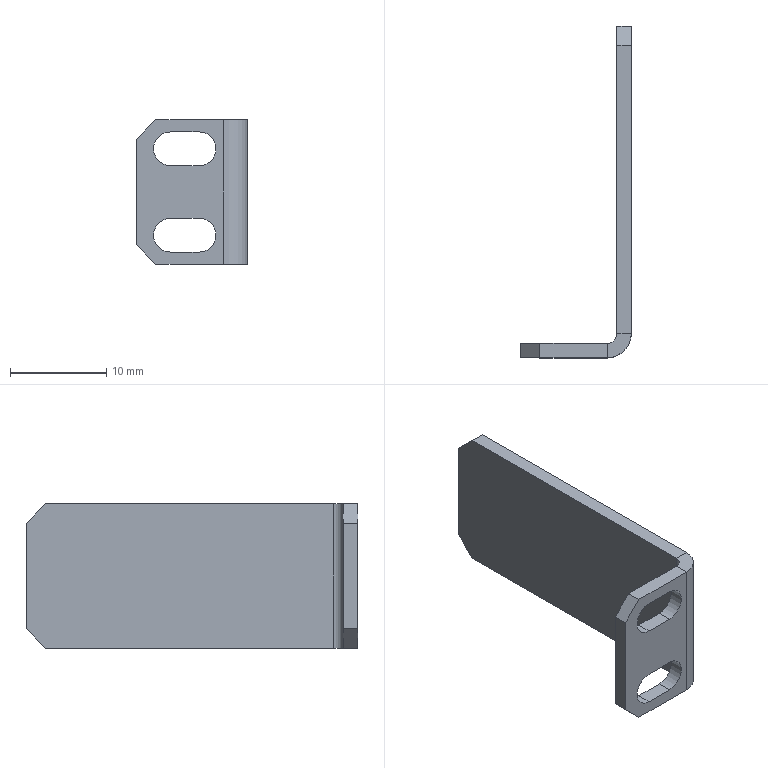Part | NX | 1 solid | 26 faces | box 11.5 x 34.5 x 15 mm | volume 911.987 mm3 | plane 20 | cylinder 6 | commonest cylinder face diameters 3.5 x4 2 x1 5 x1
STEP:
#1=CARTESIAN_POINT('',(4.,-1.5,-7.5));
#2=VERTEX_POINT('',#1);
#3=CARTESIAN_POINT('',(-3.,-1.5,-7.5));
#4=VERTEX_POINT('',#3);
#5=CARTESIAN_POINT('',(-5.,-1.5,-7.5));
#6=DIRECTION('',(-1.,0.,0.));
#7=VECTOR('',#6,1000.);
#8=LINE('',#5,#7);
#9=EDGE_CURVE('',#2,#4,#8,.T.);
#10=ORIENTED_EDGE('',*,*,#9,.T.);
#11=CARTESIAN_POINT('',(-3.,0.,-7.5));
#12=VERTEX_POINT('',#11);
#13=CARTESIAN_POINT('',(-3.,-1.5,-7.5));
#14=DIRECTION('',(0.,1.,0.));
#15=VECTOR('',#14,1000.);
#16=LINE('',#13,#15);
#17=EDGE_CURVE('',#4,#12,#16,.T.);
#18=ORIENTED_EDGE('',*,*,#17,.T.);
#19=CARTESIAN_POINT('',(4.,0.,-7.5));
#20=VERTEX_POINT('',#19);
#21=CARTESIAN_POINT('',(-5.,0.,-7.5));
#22=DIRECTION('',(-1.,0.,0.));
#23=VECTOR('',#22,1000.);
#24=LINE('',#21,#23);
#25=EDGE_CURVE('',#20,#12,#24,.T.);
#26=ORIENTED_EDGE('',*,*,#25,.F.);
#27=CARTESIAN_POINT('',(4.,0.,-7.5));
#28=DIRECTION('',(0.,-1.,0.));
#29=VECTOR('',#28,1000.);
#30=LINE('',#27,#29);
#31=EDGE_CURVE('',#20,#2,#30,.T.);
#32=ORIENTED_EDGE('',*,*,#31,.T.);
#33=EDGE_LOOP('',(#10,#18,#26,#32));
#34=FACE_BOUND('',#33,.T.);
#35=CARTESIAN_POINT('',(-5.,-1.5,-7.5));
#36=DIRECTION('',(0.,0.,-1.));
#37=DIRECTION('',(-1.,0.,0.));
#38=AXIS2_PLACEMENT_3D('',#35,#36,#37);
#39=PLANE('',#38);
#40=ADVANCED_FACE('',(#34),#39,.T.);
#41=CARTESIAN_POINT('',(-1.5,-1.5,6.25));
#42=VERTEX_POINT('',#41);
#43=CARTESIAN_POINT('',(-1.5,-1.5,2.75));
#44=VERTEX_POINT('',#43);
#45=CARTESIAN_POINT('',(-1.5,-1.5,4.5));
#46=DIRECTION('',(0.,-1.,0.));
#47=DIRECTION('',(0.,0.,-1.));
#48=AXIS2_PLACEMENT_3D('',#45,#46,#47);
#49=CIRCLE('',#48,1.75);
#50=EDGE_CURVE('',#42,#44,#49,.T.);
#51=ORIENTED_EDGE('',*,*,#50,.F.);
#52=CARTESIAN_POINT('',(1.5,-1.5,6.25));
#53=VERTEX_POINT('',#52);
#54=CARTESIAN_POINT('',(-1.5,-1.5,6.25));
#55=DIRECTION('',(-1.,0.,0.));
#56=VECTOR('',#55,1000.);
#57=LINE('',#54,#56);
#58=EDGE_CURVE('',#53,#42,#57,.T.);
#59=ORIENTED_EDGE('',*,*,#58,.F.);
#60=CARTESIAN_POINT('',(1.5,-1.5,2.75));
#61=VERTEX_POINT('',#60);
#62=CARTESIAN_POINT('',(1.5,-1.5,4.5));
#63=DIRECTION('',(0.,-1.,0.));
#64=DIRECTION('',(0.,0.,-1.));
#65=AXIS2_PLACEMENT_3D('',#62,#63,#64);
#66=CIRCLE('',#65,1.75);
#67=EDGE_CURVE('',#61,#53,#66,.T.);
#68=ORIENTED_EDGE('',*,*,#67,.F.);
#69=CARTESIAN_POINT('',(-1.5,-1.5,2.75));
#70=DIRECTION('',(1.,0.,0.));
#71=VECTOR('',#70,1000.);
#72=LINE('',#69,#71);
#73=EDGE_CURVE('',#44,#61,#72,.T.);
#74=ORIENTED_EDGE('',*,*,#73,.F.);
#75=EDGE_LOOP('',(#51,#59,#68,#74));
#76=FACE_BOUND('',#75,.T.);
#77=CARTESIAN_POINT('',(-1.5,-1.5,-2.75));
#78=VERTEX_POINT('',#77);
#79=CARTESIAN_POINT('',(-1.5,-1.5,-6.25));
#80=VERTEX_POINT('',#79);
#81=CARTESIAN_POINT('',(-1.5,-1.5,-4.5));
#82=DIRECTION('',(0.,-1.,0.));
#83=DIRECTION('',(0.,0.,-1.));
#84=AXIS2_PLACEMENT_3D('',#81,#82,#83);
#85=CIRCLE('',#84,1.75);
#86=EDGE_CURVE('',#78,#80,#85,.T.);
#87=ORIENTED_EDGE('',*,*,#86,.F.);
#88=CARTESIAN_POINT('',(1.5,-1.5,-2.75));
#89=VERTEX_POINT('',#88);
#90=CARTESIAN_POINT('',(-1.5,-1.5,-2.75));
#91=DIRECTION('',(-1.,0.,0.));
#92=VECTOR('',#91,1000.);
#93=LINE('',#90,#92);
#94=EDGE_CURVE('',#89,#78,#93,.T.);
#95=ORIENTED_EDGE('',*,*,#94,.F.);
#96=CARTESIAN_POINT('',(1.5,-1.5,-6.25));
#97=VERTEX_POINT('',#96);
#98=CARTESIAN_POINT('',(1.5,-1.5,-4.5));
#99=DIRECTION('',(0.,-1.,0.));
#100=DIRECTION('',(0.,0.,-1.));
#101=AXIS2_PLACEMENT_3D('',#98,#99,#100);
#102=CIRCLE('',#101,1.75);
#103=EDGE_CURVE('',#97,#89,#102,.T.);
#104=ORIENTED_EDGE('',*,*,#103,.F.);
#105=CARTESIAN_POINT('',(-1.5,-1.5,-6.25));
#106=DIRECTION('',(1.,0.,0.));
#107=VECTOR('',#106,1000.);
#108=LINE('',#105,#107);
#109=EDGE_CURVE('',#80,#97,#108,.T.);
#110=ORIENTED_EDGE('',*,*,#109,.F.);
#111=EDGE_LOOP('',(#87,#95,#104,#110));
#112=FACE_BOUND('',#111,.T.);
#113=CARTESIAN_POINT('',(-3.,-1.5,7.5));
#114=VERTEX_POINT('',#113);
#115=CARTESIAN_POINT('',(4.,-1.5,7.5));
#116=VERTEX_POINT('',#115);
#117=CARTESIAN_POINT('',(-5.,-1.5,7.5));
#118=DIRECTION('',(1.,0.,0.));
#119=VECTOR('',#118,1000.);
#120=LINE('',#117,#119);
#121=EDGE_CURVE('',#114,#116,#120,.T.);
#122=ORIENTED_EDGE('',*,*,#121,.F.);
#123=CARTESIAN_POINT('',(-5.,-1.5,5.5));
#124=VERTEX_POINT('',#123);
#125=CARTESIAN_POINT('',(-5.25,-1.5,5.25));
#126=DIRECTION('',(0.7071,0.,0.7071));
#127=VECTOR('',#126,1000.);
#128=LINE('',#125,#127);
#129=EDGE_CURVE('',#114,#124,#128,.F.);
#130=ORIENTED_EDGE('',*,*,#129,.T.);
#131=CARTESIAN_POINT('',(-5.,-1.5,-5.5));
#132=VERTEX_POINT('',#131);
#133=CARTESIAN_POINT('',(-5.,-1.5,7.5));
#134=DIRECTION('',(0.,0.,1.));
#135=VECTOR('',#134,1000.);
#136=LINE('',#133,#135);
#137=EDGE_CURVE('',#132,#124,#136,.T.);
#138=ORIENTED_EDGE('',*,*,#137,.F.);
#139=CARTESIAN_POINT('',(-5.25,-1.5,-5.25));
#140=DIRECTION('',(-0.7071,0.,0.7071));
#141=VECTOR('',#140,1000.);
#142=LINE('',#139,#141);
#143=EDGE_CURVE('',#132,#4,#142,.F.);
#144=ORIENTED_EDGE('',*,*,#143,.T.);
#145=ORIENTED_EDGE('',*,*,#9,.F.);
#146=CARTESIAN_POINT('',(4.,-1.5,-7.5));
#147=DIRECTION('',(0.,0.,-1.));
#148=VECTOR('',#147,1000.);
#149=LINE('',#146,#148);
#150=EDGE_CURVE('',#2,#116,#149,.F.);
#151=ORIENTED_EDGE('',*,*,#150,.T.);
#152=EDGE_LOOP('',(#122,#130,#138,#144,#145,#151));
#153=FACE_BOUND('',#152,.T.);
#154=CARTESIAN_POINT('',(0.,-1.5,0.));
#155=DIRECTION('',(0.,-1.,0.));
#156=DIRECTION('',(0.,0.,-1.));
#157=AXIS2_PLACEMENT_3D('',#154,#155,#156);
#158=PLANE('',#157);
#159=ADVANCED_FACE('',(#76,#112,#153),#158,.T.);
#160=CARTESIAN_POINT('',(1.5,0.,6.25));
#161=VERTEX_POINT('',#160);
#162=CARTESIAN_POINT('',(-1.5,0.,6.25));
#163=VERTEX_POINT('',#162);
#164=CARTESIAN_POINT('',(0.,0.,6.25));
#165=DIRECTION('',(-1.,0.,0.));
#166=VECTOR('',#165,1000.);
#167=LINE('',#164,#166);
#168=EDGE_CURVE('',#161,#163,#167,.T.);
#169=ORIENTED_EDGE('',*,*,#168,.T.);
#170=CARTESIAN_POINT('',(-1.5,0.,2.75));
#171=VERTEX_POINT('',#170);
#172=CARTESIAN_POINT('',(-1.5,0.,4.5));
#173=DIRECTION('',(0.,-1.,0.));
#174=DIRECTION('',(0.,0.,-1.));
#175=AXIS2_PLACEMENT_3D('',#172,#173,#174);
#176=CIRCLE('',#175,1.75);
#177=EDGE_CURVE('',#163,#171,#176,.T.);
#178=ORIENTED_EDGE('',*,*,#177,.T.);
#179=CARTESIAN_POINT('',(1.5,0.,2.75));
#180=VERTEX_POINT('',#179);
#181=CARTESIAN_POINT('',(0.,0.,2.75));
#182=DIRECTION('',(1.,0.,0.));
#183=VECTOR('',#182,1000.);
#184=LINE('',#181,#183);
#185=EDGE_CURVE('',#171,#180,#184,.T.);
#186=ORIENTED_EDGE('',*,*,#185,.T.);
#187=CARTESIAN_POINT('',(1.5,0.,4.5));
#188=DIRECTION('',(0.,-1.,0.));
#189=DIRECTION('',(0.,0.,-1.));
#190=AXIS2_PLACEMENT_3D('',#187,#188,#189);
#191=CIRCLE('',#190,1.75);
#192=EDGE_CURVE('',#180,#161,#191,.T.);
#193=ORIENTED_EDGE('',*,*,#192,.T.);
#194=EDGE_LOOP('',(#169,#178,#186,#193));
#195=FACE_BOUND('',#194,.T.);
#196=CARTESIAN_POINT('',(1.5,0.,-2.75));
#197=VERTEX_POINT('',#196);
#198=CARTESIAN_POINT('',(-1.5,0.,-2.75));
#199=VERTEX_POINT('',#198);
#200=CARTESIAN_POINT('',(0.,0.,-2.75));
#201=DIRECTION('',(-1.,0.,0.));
#202=VECTOR('',#201,1000.);
#203=LINE('',#200,#202);
#204=EDGE_CURVE('',#197,#199,#203,.T.);
#205=ORIENTED_EDGE('',*,*,#204,.T.);
#206=CARTESIAN_POINT('',(-1.5,0.,-6.25));
#207=VERTEX_POINT('',#206);
#208=CARTESIAN_POINT('',(-1.5,0.,-4.5));
#209=DIRECTION('',(0.,-1.,0.));
#210=DIRECTION('',(0.,0.,-1.));
#211=AXIS2_PLACEMENT_3D('',#208,#209,#210);
#212=CIRCLE('',#211,1.75);
#213=EDGE_CURVE('',#199,#207,#212,.T.);
#214=ORIENTED_EDGE('',*,*,#213,.T.);
#215=CARTESIAN_POINT('',(1.5,0.,-6.25));
#216=VERTEX_POINT('',#215);
#217=CARTESIAN_POINT('',(0.,0.,-6.25));
#218=DIRECTION('',(1.,0.,0.));
#219=VECTOR('',#218,1000.);
#220=LINE('',#217,#219);
#221=EDGE_CURVE('',#207,#216,#220,.T.);
#222=ORIENTED_EDGE('',*,*,#221,.T.);
#223=CARTESIAN_POINT('',(1.5,0.,-4.5));
#224=DIRECTION('',(0.,-1.,0.));
#225=DIRECTION('',(0.,0.,-1.));
#226=AXIS2_PLACEMENT_3D('',#223,#224,#225);
#227=CIRCLE('',#226,1.75);
#228=EDGE_CURVE('',#216,#197,#227,.T.);
#229=ORIENTED_EDGE('',*,*,#228,.T.);
#230=EDGE_LOOP('',(#205,#214,#222,#229));
#231=FACE_BOUND('',#230,.T.);
#232=CARTESIAN_POINT('',(-5.,0.,-5.5));
#233=VERTEX_POINT('',#232);
#234=CARTESIAN_POINT('',(-5.,0.,5.5));
#235=VERTEX_POINT('',#234);
#236=CARTESIAN_POINT('',(-5.,0.,7.5));
#237=DIRECTION('',(0.,0.,1.));
#238=VECTOR('',#237,1000.);
#239=LINE('',#236,#238);
#240=EDGE_CURVE('',#233,#235,#239,.T.);
#241=ORIENTED_EDGE('',*,*,#240,.T.);
#242=CARTESIAN_POINT('',(-3.,0.,7.5));
#243=VERTEX_POINT('',#242);
#244=CARTESIAN_POINT('',(-5.,0.,5.5));
#245=DIRECTION('',(-0.7071,0.,-0.7071));
#246=VECTOR('',#245,1000.);
#247=LINE('',#244,#246);
#248=EDGE_CURVE('',#235,#243,#247,.F.);
#249=ORIENTED_EDGE('',*,*,#248,.T.);
#250=CARTESIAN_POINT('',(4.,0.,7.5));
#251=VERTEX_POINT('',#250);
#252=CARTESIAN_POINT('',(-5.,0.,7.5));
#253=DIRECTION('',(1.,0.,0.));
#254=VECTOR('',#253,1000.);
#255=LINE('',#252,#254);
#256=EDGE_CURVE('',#243,#251,#255,.T.);
#257=ORIENTED_EDGE('',*,*,#256,.T.);
#258=CARTESIAN_POINT('',(4.,0.,-7.5));
#259=DIRECTION('',(0.,0.,-1.));
#260=VECTOR('',#259,1000.);
#261=LINE('',#258,#260);
#262=EDGE_CURVE('',#20,#251,#261,.F.);
#263=ORIENTED_EDGE('',*,*,#262,.F.);
#264=ORIENTED_EDGE('',*,*,#25,.T.);
#265=CARTESIAN_POINT('',(-3.,0.,-7.5));
#266=DIRECTION('',(0.7071,0.,-0.7071));
#267=VECTOR('',#266,1000.);
#268=LINE('',#265,#267);
#269=EDGE_CURVE('',#12,#233,#268,.F.);
#270=ORIENTED_EDGE('',*,*,#269,.T.);
#271=EDGE_LOOP('',(#241,#249,#257,#263,#264,#270));
#272=FACE_BOUND('',#271,.T.);
#273=CARTESIAN_POINT('',(0.,0.,0.));
#274=DIRECTION('',(0.,-1.,0.));
#275=DIRECTION('',(0.,0.,-1.));
#276=AXIS2_PLACEMENT_3D('',#273,#274,#275);
#277=PLANE('',#276);
#278=ADVANCED_FACE('',(#195,#231,#272),#277,.F.);
#279=ORIENTED_EDGE('',*,*,#256,.F.);
#280=CARTESIAN_POINT('',(-3.,-1.5,7.5));
#281=DIRECTION('',(0.,-1.,0.));
#282=VECTOR('',#281,1000.);
#283=LINE('',#280,#282);
#284=EDGE_CURVE('',#243,#114,#283,.T.);
#285=ORIENTED_EDGE('',*,*,#284,.T.);
#286=ORIENTED_EDGE('',*,*,#121,.T.);
#287=CARTESIAN_POINT('',(4.,0.,7.5));
#288=DIRECTION('',(0.,-1.,0.));
#289=VECTOR('',#288,1000.);
#290=LINE('',#287,#289);
#291=EDGE_CURVE('',#251,#116,#290,.T.);
#292=ORIENTED_EDGE('',*,*,#291,.F.);
#293=EDGE_LOOP('',(#279,#285,#286,#292));
#294=FACE_BOUND('',#293,.T.);
#295=CARTESIAN_POINT('',(-5.,-1.5,7.5));
#296=DIRECTION('',(0.,0.,1.));
#297=DIRECTION('',(1.,0.,0.));
#298=AXIS2_PLACEMENT_3D('',#295,#296,#297);
#299=PLANE('',#298);
#300=ADVANCED_FACE('',(#294),#299,.T.);
#301=ORIENTED_EDGE('',*,*,#137,.T.);
#302=CARTESIAN_POINT('',(-5.,-1.5,5.5));
#303=DIRECTION('',(0.,1.,0.));
#304=VECTOR('',#303,1000.);
#305=LINE('',#302,#304);
#306=EDGE_CURVE('',#124,#235,#305,.T.);
#307=ORIENTED_EDGE('',*,*,#306,.T.);
#308=ORIENTED_EDGE('',*,*,#240,.F.);
#309=CARTESIAN_POINT('',(-5.,-1.5,-5.5));
#310=DIRECTION('',(0.,-1.,0.));
#311=VECTOR('',#310,1000.);
#312=LINE('',#309,#311);
#313=EDGE_CURVE('',#233,#132,#312,.T.);
#314=ORIENTED_EDGE('',*,*,#313,.T.);
#315=EDGE_LOOP('',(#301,#307,#308,#314));
#316=FACE_BOUND('',#315,.T.);
#317=CARTESIAN_POINT('',(-5.,-1.5,7.5));
#318=DIRECTION('',(-1.,0.,0.));
#319=DIRECTION('',(0.,0.,1.));
#320=AXIS2_PLACEMENT_3D('',#317,#318,#319);
#321=PLANE('',#320);
#322=ADVANCED_FACE('',(#316),#321,.T.);
#323=CARTESIAN_POINT('',(5.,1.,7.5));
#324=VERTEX_POINT('',#323);
#325=CARTESIAN_POINT('',(6.5,1.,7.5));
#326=VERTEX_POINT('',#325);
#327=CARTESIAN_POINT('',(5.,1.,7.5));
#328=DIRECTION('',(1.,0.,0.));
#329=VECTOR('',#328,1000.);
#330=LINE('',#327,#329);
#331=EDGE_CURVE('',#324,#326,#330,.T.);
#332=ORIENTED_EDGE('',*,*,#331,.F.);
#333=CARTESIAN_POINT('',(4.,1.,7.5));
#334=DIRECTION('',(0.,0.,-1.));
#335=DIRECTION('',(-1.,0.,0.));
#336=AXIS2_PLACEMENT_3D('',#333,#334,#335);
#337=CIRCLE('',#336,1.);
#338=EDGE_CURVE('',#251,#324,#337,.F.);
#339=ORIENTED_EDGE('',*,*,#338,.F.);
#340=ORIENTED_EDGE('',*,*,#291,.T.);
#341=CARTESIAN_POINT('',(4.,1.,7.5));
#342=DIRECTION('',(0.,0.,-1.));
#343=DIRECTION('',(-1.,0.,0.));
#344=AXIS2_PLACEMENT_3D('',#341,#342,#343);
#345=CIRCLE('',#344,2.5);
#346=EDGE_CURVE('',#116,#326,#345,.F.);
#347=ORIENTED_EDGE('',*,*,#346,.T.);
#348=EDGE_LOOP('',(#332,#339,#340,#347));
#349=FACE_BOUND('',#348,.T.);
#350=CARTESIAN_POINT('',(4.,1.,7.5));
#351=DIRECTION('',(0.,0.,1.));
#352=DIRECTION('',(1.,0.,0.));
#353=AXIS2_PLACEMENT_3D('',#350,#351,#352);
#354=PLANE('',#353);
#355=ADVANCED_FACE('',(#349),#354,.T.);
#356=CARTESIAN_POINT('',(5.,1.,-7.5));
#357=VERTEX_POINT('',#356);
#358=CARTESIAN_POINT('',(4.,1.,-7.5));
#359=DIRECTION('',(0.,0.,-1.));
#360=DIRECTION('',(-1.,0.,0.));
#361=AXIS2_PLACEMENT_3D('',#358,#359,#360);
#362=CIRCLE('',#361,1.);
#363=EDGE_CURVE('',#357,#20,#362,.T.);
#364=ORIENTED_EDGE('',*,*,#363,.F.);
#365=CARTESIAN_POINT('',(6.5,1.,-7.5));
#366=VERTEX_POINT('',#365);
#367=CARTESIAN_POINT('',(5.,1.,-7.5));
#368=DIRECTION('',(1.,0.,0.));
#369=VECTOR('',#368,1000.);
#370=LINE('',#367,#369);
#371=EDGE_CURVE('',#357,#366,#370,.T.);
#372=ORIENTED_EDGE('',*,*,#371,.T.);
#373=CARTESIAN_POINT('',(4.,1.,-7.5));
#374=DIRECTION('',(0.,0.,-1.));
#375=DIRECTION('',(-1.,0.,0.));
#376=AXIS2_PLACEMENT_3D('',#373,#374,#375);
#377=CIRCLE('',#376,2.5);
#378=EDGE_CURVE('',#366,#2,#377,.T.);
#379=ORIENTED_EDGE('',*,*,#378,.T.);
#380=ORIENTED_EDGE('',*,*,#31,.F.);
#381=EDGE_LOOP('',(#364,#372,#379,#380));
#382=FACE_BOUND('',#381,.T.);
#383=CARTESIAN_POINT('',(4.,1.,-7.5));
#384=DIRECTION('',(0.,0.,1.));
#385=DIRECTION('',(1.,0.,0.));
#386=AXIS2_PLACEMENT_3D('',#383,#384,#385);
#387=PLANE('',#386);
#388=ADVANCED_FACE('',(#382),#387,.F.);
#389=ORIENTED_EDGE('',*,*,#150,.F.);
#390=ORIENTED_EDGE('',*,*,#378,.F.);
#391=CARTESIAN_POINT('',(6.5,1.,0.));
#392=DIRECTION('',(0.,0.,1.));
#393=VECTOR('',#392,1000.);
#394=LINE('',#391,#393);
#395=EDGE_CURVE('',#366,#326,#394,.T.);
#396=ORIENTED_EDGE('',*,*,#395,.T.);
#397=ORIENTED_EDGE('',*,*,#346,.F.);
#398=EDGE_LOOP('',(#389,#390,#396,#397));
#399=FACE_BOUND('',#398,.T.);
#400=CARTESIAN_POINT('',(4.,1.,-7.5));
#401=DIRECTION('',(0.,0.,-1.));
#402=DIRECTION('',(1.,0.,0.));
#403=AXIS2_PLACEMENT_3D('',#400,#401,#402);
#404=CYLINDRICAL_SURFACE('',#403,2.5);
#405=ADVANCED_FACE('',(#399),#404,.T.);
#406=ORIENTED_EDGE('',*,*,#262,.T.);
#407=ORIENTED_EDGE('',*,*,#338,.T.);
#408=CARTESIAN_POINT('',(5.,1.,7.5));
#409=DIRECTION('',(0.,0.,-1.));
#410=VECTOR('',#409,1000.);
#411=LINE('',#408,#410);
#412=EDGE_CURVE('',#324,#357,#411,.T.);
#413=ORIENTED_EDGE('',*,*,#412,.T.);
#414=ORIENTED_EDGE('',*,*,#363,.T.);
#415=EDGE_LOOP('',(#406,#407,#413,#414));
#416=FACE_BOUND('',#415,.T.);
#417=CARTESIAN_POINT('',(4.,1.,-7.5));
#418=DIRECTION('',(0.,0.,-1.));
#419=DIRECTION('',(1.,0.,0.));
#420=AXIS2_PLACEMENT_3D('',#417,#418,#419);
#421=CYLINDRICAL_SURFACE('',#420,1.);
#422=ADVANCED_FACE('',(#416),#421,.F.);
#423=CARTESIAN_POINT('',(6.5,31.,7.5));
#424=VERTEX_POINT('',#423);
#425=CARTESIAN_POINT('',(6.5,0.,7.5));
#426=DIRECTION('',(0.,-1.,0.));
#427=VECTOR('',#426,1000.);
#428=LINE('',#425,#427);
#429=EDGE_CURVE('',#424,#326,#428,.T.);
#430=ORIENTED_EDGE('',*,*,#429,.F.);
#431=CARTESIAN_POINT('',(5.,31.,7.5));
#432=VERTEX_POINT('',#431);
#433=CARTESIAN_POINT('',(6.5,31.,7.5));
#434=DIRECTION('',(-1.,0.,0.));
#435=VECTOR('',#434,1000.);
#436=LINE('',#433,#435);
#437=EDGE_CURVE('',#424,#432,#436,.T.);
#438=ORIENTED_EDGE('',*,*,#437,.T.);
#439=CARTESIAN_POINT('',(5.,0.,7.5));
#440=DIRECTION('',(0.,-1.,0.));
#441=VECTOR('',#440,1000.);
#442=LINE('',#439,#441);
#443=EDGE_CURVE('',#432,#324,#442,.T.);
#444=ORIENTED_EDGE('',*,*,#443,.T.);
#445=ORIENTED_EDGE('',*,*,#331,.T.);
#446=EDGE_LOOP('',(#430,#438,#444,#445));
#447=FACE_BOUND('',#446,.T.);
#448=CARTESIAN_POINT('',(6.5,0.,7.5));
#449=DIRECTION('',(0.,0.,-1.));
#450=DIRECTION('',(0.,1.,0.));
#451=AXIS2_PLACEMENT_3D('',#448,#449,#450);
#452=PLANE('',#451);
#453=ADVANCED_FACE('',(#447),#452,.F.);
#454=CARTESIAN_POINT('',(5.,31.,-7.5));
#455=VERTEX_POINT('',#454);
#456=CARTESIAN_POINT('',(5.,33.,-7.5));
#457=DIRECTION('',(0.,1.,0.));
#458=VECTOR('',#457,1000.);
#459=LINE('',#456,#458);
#460=EDGE_CURVE('',#357,#455,#459,.T.);
#461=ORIENTED_EDGE('',*,*,#460,.T.);
#462=CARTESIAN_POINT('',(6.5,31.,-7.5));
#463=VERTEX_POINT('',#462);
#464=CARTESIAN_POINT('',(6.5,31.,-7.5));
#465=DIRECTION('',(1.,0.,0.));
#466=VECTOR('',#465,1000.);
#467=LINE('',#464,#466);
#468=EDGE_CURVE('',#455,#463,#467,.T.);
#469=ORIENTED_EDGE('',*,*,#468,.T.);
#470=CARTESIAN_POINT('',(6.5,33.,-7.5));
#471=DIRECTION('',(0.,1.,0.));
#472=VECTOR('',#471,1000.);
#473=LINE('',#470,#472);
#474=EDGE_CURVE('',#366,#463,#473,.T.);
#475=ORIENTED_EDGE('',*,*,#474,.F.);
#476=ORIENTED_EDGE('',*,*,#371,.F.);
#477=EDGE_LOOP('',(#461,#469,#475,#476));
#478=FACE_BOUND('',#477,.T.);
#479=CARTESIAN_POINT('',(6.5,33.,-7.5));
#480=DIRECTION('',(0.,0.,1.));
#481=DIRECTION('',(0.,-1.,0.));
#482=AXIS2_PLACEMENT_3D('',#479,#480,#481);
#483=PLANE('',#482);
#484=ADVANCED_FACE('',(#478),#483,.F.);
#485=CARTESIAN_POINT('',(6.5,33.,-5.5));
#486=VERTEX_POINT('',#485);
#487=CARTESIAN_POINT('',(6.5,33.,5.5));
#488=VERTEX_POINT('',#487);
#489=CARTESIAN_POINT('',(6.5,33.,7.5));
#490=DIRECTION('',(0.,0.,1.));
#491=VECTOR('',#490,1000.);
#492=LINE('',#489,#491);
#493=EDGE_CURVE('',#486,#488,#492,.T.);
#494=ORIENTED_EDGE('',*,*,#493,.T.);
#495=CARTESIAN_POINT('',(6.5,31.,7.5));
#496=DIRECTION('',(0.,0.7071,-0.7071));
#497=VECTOR('',#496,1000.);
#498=LINE('',#495,#497);
#499=EDGE_CURVE('',#488,#424,#498,.F.);
#500=ORIENTED_EDGE('',*,*,#499,.T.);
#501=ORIENTED_EDGE('',*,*,#429,.T.);
#502=ORIENTED_EDGE('',*,*,#395,.F.);
#503=ORIENTED_EDGE('',*,*,#474,.T.);
#504=CARTESIAN_POINT('',(6.5,33.,-5.5));
#505=DIRECTION('',(0.,-0.7071,-0.7071));
#506=VECTOR('',#505,1000.);
#507=LINE('',#504,#506);
#508=EDGE_CURVE('',#463,#486,#507,.F.);
#509=ORIENTED_EDGE('',*,*,#508,.T.);
#510=EDGE_LOOP('',(#494,#500,#501,#502,#503,#509));
#511=FACE_BOUND('',#510,.T.);
#512=CARTESIAN_POINT('',(6.5,0.,0.));
#513=DIRECTION('',(-1.,0.,0.));
#514=DIRECTION('',(0.,-1.,0.));
#515=AXIS2_PLACEMENT_3D('',#512,#513,#514);
#516=PLANE('',#515);
#517=ADVANCED_FACE('',(#511),#516,.F.);
#518=ORIENTED_EDGE('',*,*,#443,.F.);
#519=CARTESIAN_POINT('',(5.,33.,5.5));
#520=VERTEX_POINT('',#519);
#521=CARTESIAN_POINT('',(5.,19.25,19.25));
#522=DIRECTION('',(0.,-0.7071,0.7071));
#523=VECTOR('',#522,1000.);
#524=LINE('',#521,#523);
#525=EDGE_CURVE('',#432,#520,#524,.F.);
#526=ORIENTED_EDGE('',*,*,#525,.T.);
#527=CARTESIAN_POINT('',(5.,33.,-5.5));
#528=VERTEX_POINT('',#527);
#529=CARTESIAN_POINT('',(5.,33.,7.5));
#530=DIRECTION('',(0.,0.,1.));
#531=VECTOR('',#530,1000.);
#532=LINE('',#529,#531);
#533=EDGE_CURVE('',#528,#520,#532,.T.);
#534=ORIENTED_EDGE('',*,*,#533,.F.);
#535=CARTESIAN_POINT('',(5.,19.25,-19.25));
#536=DIRECTION('',(0.,0.7071,0.7071));
#537=VECTOR('',#536,1000.);
#538=LINE('',#535,#537);
#539=EDGE_CURVE('',#528,#455,#538,.F.);
#540=ORIENTED_EDGE('',*,*,#539,.T.);
#541=ORIENTED_EDGE('',*,*,#460,.F.);
#542=ORIENTED_EDGE('',*,*,#412,.F.);
#543=EDGE_LOOP('',(#518,#526,#534,#540,#541,#542));
#544=FACE_BOUND('',#543,.T.);
#545=CARTESIAN_POINT('',(5.,0.,0.));
#546=DIRECTION('',(-1.,0.,0.));
#547=DIRECTION('',(0.,-1.,0.));
#548=AXIS2_PLACEMENT_3D('',#545,#546,#547);
#549=PLANE('',#548);
#550=ADVANCED_FACE('',(#544),#549,.T.);
#551=ORIENTED_EDGE('',*,*,#533,.T.);
#552=CARTESIAN_POINT('',(6.5,33.,5.5));
#553=DIRECTION('',(1.,0.,0.));
#554=VECTOR('',#553,1000.);
#555=LINE('',#552,#554);
#556=EDGE_CURVE('',#520,#488,#555,.T.);
#557=ORIENTED_EDGE('',*,*,#556,.T.);
#558=ORIENTED_EDGE('',*,*,#493,.F.);
#559=CARTESIAN_POINT('',(6.5,33.,-5.5));
#560=DIRECTION('',(-1.,0.,0.));
#561=VECTOR('',#560,1000.);
#562=LINE('',#559,#561);
#563=EDGE_CURVE('',#486,#528,#562,.T.);
#564=ORIENTED_EDGE('',*,*,#563,.T.);
#565=EDGE_LOOP('',(#551,#557,#558,#564));
#566=FACE_BOUND('',#565,.T.);
#567=CARTESIAN_POINT('',(6.5,33.,7.5));
#568=DIRECTION('',(0.,-1.,0.));
#569=DIRECTION('',(1.,0.,0.));
#570=AXIS2_PLACEMENT_3D('',#567,#568,#569);
#571=PLANE('',#570);
#572=ADVANCED_FACE('',(#566),#571,.F.);
#573=ORIENTED_EDGE('',*,*,#129,.F.);
#574=ORIENTED_EDGE('',*,*,#284,.F.);
#575=ORIENTED_EDGE('',*,*,#248,.F.);
#576=ORIENTED_EDGE('',*,*,#306,.F.);
#577=EDGE_LOOP('',(#573,#574,#575,#576));
#578=FACE_BOUND('',#577,.T.);
#579=CARTESIAN_POINT('',(-5.,-1.5,5.5));
#580=DIRECTION('',(0.7071,0.,-0.7071));
#581=DIRECTION('',(0.,1.,0.));
#582=AXIS2_PLACEMENT_3D('',#579,#580,#581);
#583=PLANE('',#582);
#584=ADVANCED_FACE('',(#578),#583,.F.);
#585=ORIENTED_EDGE('',*,*,#143,.F.);
#586=ORIENTED_EDGE('',*,*,#313,.F.);
#587=ORIENTED_EDGE('',*,*,#269,.F.);
#588=ORIENTED_EDGE('',*,*,#17,.F.);
#589=EDGE_LOOP('',(#585,#586,#587,#588));
#590=FACE_BOUND('',#589,.T.);
#591=CARTESIAN_POINT('',(-3.,-1.5,-7.5));
#592=DIRECTION('',(0.7071,0.,0.7071));
#593=DIRECTION('',(0.,1.,0.));
#594=AXIS2_PLACEMENT_3D('',#591,#592,#593);
#595=PLANE('',#594);
#596=ADVANCED_FACE('',(#590),#595,.F.);
#597=CARTESIAN_POINT('',(-1.5,33.,-2.75));
#598=DIRECTION('',(0.,-1.,0.));
#599=VECTOR('',#598,1000.);
#600=LINE('',#597,#599);
#601=EDGE_CURVE('',#199,#78,#600,.T.);
#602=ORIENTED_EDGE('',*,*,#601,.T.);
#603=ORIENTED_EDGE('',*,*,#86,.T.);
#604=CARTESIAN_POINT('',(-1.5,33.,-6.25));
#605=DIRECTION('',(0.,-1.,0.));
#606=VECTOR('',#605,1000.);
#607=LINE('',#604,#606);
#608=EDGE_CURVE('',#207,#80,#607,.T.);
#609=ORIENTED_EDGE('',*,*,#608,.F.);
#610=ORIENTED_EDGE('',*,*,#213,.F.);
#611=EDGE_LOOP('',(#602,#603,#609,#610));
#612=FACE_BOUND('',#611,.T.);
#613=CARTESIAN_POINT('',(-1.5,33.,-4.5));
#614=DIRECTION('',(0.,-1.,0.));
#615=DIRECTION('',(0.,0.,-1.));
#616=AXIS2_PLACEMENT_3D('',#613,#614,#615);
#617=CYLINDRICAL_SURFACE('',#616,1.75);
#618=ADVANCED_FACE('',(#612),#617,.F.);
#619=CARTESIAN_POINT('',(1.5,33.,-2.75));
#620=DIRECTION('',(0.,-1.,0.));
#621=VECTOR('',#620,1000.);
#622=LINE('',#619,#621);
#623=EDGE_CURVE('',#197,#89,#622,.T.);
#624=ORIENTED_EDGE('',*,*,#623,.T.);
#625=ORIENTED_EDGE('',*,*,#94,.T.);
#626=ORIENTED_EDGE('',*,*,#601,.F.);
#627=ORIENTED_EDGE('',*,*,#204,.F.);
#628=EDGE_LOOP('',(#624,#625,#626,#627));
#629=FACE_BOUND('',#628,.T.);
#630=CARTESIAN_POINT('',(-1.5,33.,-2.75));
#631=DIRECTION('',(0.,0.,1.));
#632=DIRECTION('',(1.,0.,0.));
#633=AXIS2_PLACEMENT_3D('',#630,#631,#632);
#634=PLANE('',#633);
#635=ADVANCED_FACE('',(#629),#634,.F.);
#636=CARTESIAN_POINT('',(1.5,33.,-6.25));
#637=DIRECTION('',(0.,-1.,0.));
#638=VECTOR('',#637,1000.);
#639=LINE('',#636,#638);
#640=EDGE_CURVE('',#216,#97,#639,.T.);
#641=ORIENTED_EDGE('',*,*,#640,.T.);
#642=ORIENTED_EDGE('',*,*,#103,.T.);
#643=ORIENTED_EDGE('',*,*,#623,.F.);
#644=ORIENTED_EDGE('',*,*,#228,.F.);
#645=EDGE_LOOP('',(#641,#642,#643,#644));
#646=FACE_BOUND('',#645,.T.);
#647=CARTESIAN_POINT('',(1.5,33.,-4.5));
#648=DIRECTION('',(0.,-1.,0.));
#649=DIRECTION('',(0.,0.,-1.));
#650=AXIS2_PLACEMENT_3D('',#647,#648,#649);
#651=CYLINDRICAL_SURFACE('',#650,1.75);
#652=ADVANCED_FACE('',(#646),#651,.F.);
#653=ORIENTED_EDGE('',*,*,#608,.T.);
#654=ORIENTED_EDGE('',*,*,#109,.T.);
#655=ORIENTED_EDGE('',*,*,#640,.F.);
#656=ORIENTED_EDGE('',*,*,#221,.F.);
#657=EDGE_LOOP('',(#653,#654,#655,#656));
#658=FACE_BOUND('',#657,.T.);
#659=CARTESIAN_POINT('',(-1.5,33.,-6.25));
#660=DIRECTION('',(0.,0.,-1.));
#661=DIRECTION('',(-1.,0.,0.));
#662=AXIS2_PLACEMENT_3D('',#659,#660,#661);
#663=PLANE('',#662);
#664=ADVANCED_FACE('',(#658),#663,.F.);
#665=CARTESIAN_POINT('',(-1.5,33.,6.25));
#666=DIRECTION('',(0.,-1.,0.));
#667=VECTOR('',#666,1000.);
#668=LINE('',#665,#667);
#669=EDGE_CURVE('',#163,#42,#668,.T.);
#670=ORIENTED_EDGE('',*,*,#669,.T.);
#671=ORIENTED_EDGE('',*,*,#50,.T.);
#672=CARTESIAN_POINT('',(-1.5,33.,2.75));
#673=DIRECTION('',(0.,-1.,0.));
#674=VECTOR('',#673,1000.);
#675=LINE('',#672,#674);
#676=EDGE_CURVE('',#171,#44,#675,.T.);
#677=ORIENTED_EDGE('',*,*,#676,.F.);
#678=ORIENTED_EDGE('',*,*,#177,.F.);
#679=EDGE_LOOP('',(#670,#671,#677,#678));
#680=FACE_BOUND('',#679,.T.);
#681=CARTESIAN_POINT('',(-1.5,33.,4.5));
#682=DIRECTION('',(0.,-1.,0.));
#683=DIRECTION('',(0.,0.,-1.));
#684=AXIS2_PLACEMENT_3D('',#681,#682,#683);
#685=CYLINDRICAL_SURFACE('',#684,1.75);
#686=ADVANCED_FACE('',(#680),#685,.F.);
#687=CARTESIAN_POINT('',(1.5,33.,6.25));
#688=DIRECTION('',(0.,-1.,0.));
#689=VECTOR('',#688,1000.);
#690=LINE('',#687,#689);
#691=EDGE_CURVE('',#161,#53,#690,.T.);
#692=ORIENTED_EDGE('',*,*,#691,.T.);
#693=ORIENTED_EDGE('',*,*,#58,.T.);
#694=ORIENTED_EDGE('',*,*,#669,.F.);
#695=ORIENTED_EDGE('',*,*,#168,.F.);
#696=EDGE_LOOP('',(#692,#693,#694,#695));
#697=FACE_BOUND('',#696,.T.);
#698=CARTESIAN_POINT('',(-1.5,33.,6.25));
#699=DIRECTION('',(0.,0.,1.));
#700=DIRECTION('',(1.,0.,0.));
#701=AXIS2_PLACEMENT_3D('',#698,#699,#700);
#702=PLANE('',#701);
#703=ADVANCED_FACE('',(#697),#702,.F.);
#704=CARTESIAN_POINT('',(1.5,33.,2.75));
#705=DIRECTION('',(0.,-1.,0.));
#706=VECTOR('',#705,1000.);
#707=LINE('',#704,#706);
#708=EDGE_CURVE('',#180,#61,#707,.T.);
#709=ORIENTED_EDGE('',*,*,#708,.T.);
#710=ORIENTED_EDGE('',*,*,#67,.T.);
#711=ORIENTED_EDGE('',*,*,#691,.F.);
#712=ORIENTED_EDGE('',*,*,#192,.F.);
#713=EDGE_LOOP('',(#709,#710,#711,#712));
#714=FACE_BOUND('',#713,.T.);
#715=CARTESIAN_POINT('',(1.5,33.,4.5));
#716=DIRECTION('',(0.,-1.,0.));
#717=DIRECTION('',(0.,0.,-1.));
#718=AXIS2_PLACEMENT_3D('',#715,#716,#717);
#719=CYLINDRICAL_SURFACE('',#718,1.75);
#720=ADVANCED_FACE('',(#714),#719,.F.);
#721=ORIENTED_EDGE('',*,*,#676,.T.);
#722=ORIENTED_EDGE('',*,*,#73,.T.);
#723=ORIENTED_EDGE('',*,*,#708,.F.);
#724=ORIENTED_EDGE('',*,*,#185,.F.);
#725=EDGE_LOOP('',(#721,#722,#723,#724));
#726=FACE_BOUND('',#725,.T.);
#727=CARTESIAN_POINT('',(-1.5,33.,2.75));
#728=DIRECTION('',(0.,0.,-1.));
#729=DIRECTION('',(-1.,0.,0.));
#730=AXIS2_PLACEMENT_3D('',#727,#728,#729);
#731=PLANE('',#730);
#732=ADVANCED_FACE('',(#726),#731,.F.);
#733=ORIENTED_EDGE('',*,*,#499,.F.);
#734=ORIENTED_EDGE('',*,*,#556,.F.);
#735=ORIENTED_EDGE('',*,*,#525,.F.);
#736=ORIENTED_EDGE('',*,*,#437,.F.);
#737=EDGE_LOOP('',(#733,#734,#735,#736));
#738=FACE_BOUND('',#737,.T.);
#739=CARTESIAN_POINT('',(6.5,31.,7.5));
#740=DIRECTION('',(0.,-0.7071,-0.7071));
#741=DIRECTION('',(-1.,0.,0.));
#742=AXIS2_PLACEMENT_3D('',#739,#740,#741);
#743=PLANE('',#742);
#744=ADVANCED_FACE('',(#738),#743,.F.);
#745=ORIENTED_EDGE('',*,*,#508,.F.);
#746=ORIENTED_EDGE('',*,*,#468,.F.);
#747=ORIENTED_EDGE('',*,*,#539,.F.);
#748=ORIENTED_EDGE('',*,*,#563,.F.);
#749=EDGE_LOOP('',(#745,#746,#747,#748));
#750=FACE_BOUND('',#749,.T.);
#751=CARTESIAN_POINT('',(6.5,33.,-5.5));
#752=DIRECTION('',(0.,-0.7071,0.7071));
#753=DIRECTION('',(-1.,0.,0.));
#754=AXIS2_PLACEMENT_3D('',#751,#752,#753);
#755=PLANE('',#754);
#756=ADVANCED_FACE('',(#750),#755,.F.);
#757=CLOSED_SHELL('',(#40,#159,#278,#300,#322,#355,#388,#405,#422,#453,#484,#517,#550,#572,#584,#596,#618,#635,#652,#664,#686,#703,#720,#732,#744,#756));
#758=MANIFOLD_SOLID_BREP('',#757);
#759=(LENGTH_UNIT()NAMED_UNIT(*)SI_UNIT(.MILLI.,.METRE.));
#760=UNCERTAINTY_MEASURE_WITH_UNIT(LENGTH_MEASURE(0.00001),#759,'','');
#761=(NAMED_UNIT(*)PLANE_ANGLE_UNIT()SI_UNIT($,.RADIAN.));
#762=(NAMED_UNIT(*)SI_UNIT($,.STERADIAN.)SOLID_ANGLE_UNIT());
#763=(GEOMETRIC_REPRESENTATION_CONTEXT(3)GLOBAL_UNCERTAINTY_ASSIGNED_CONTEXT((#760))GLOBAL_UNIT_ASSIGNED_CONTEXT((#759,#761,#762))REPRESENTATION_CONTEXT('',''));
#764=ADVANCED_BREP_SHAPE_REPRESENTATION('',(#758),#763);